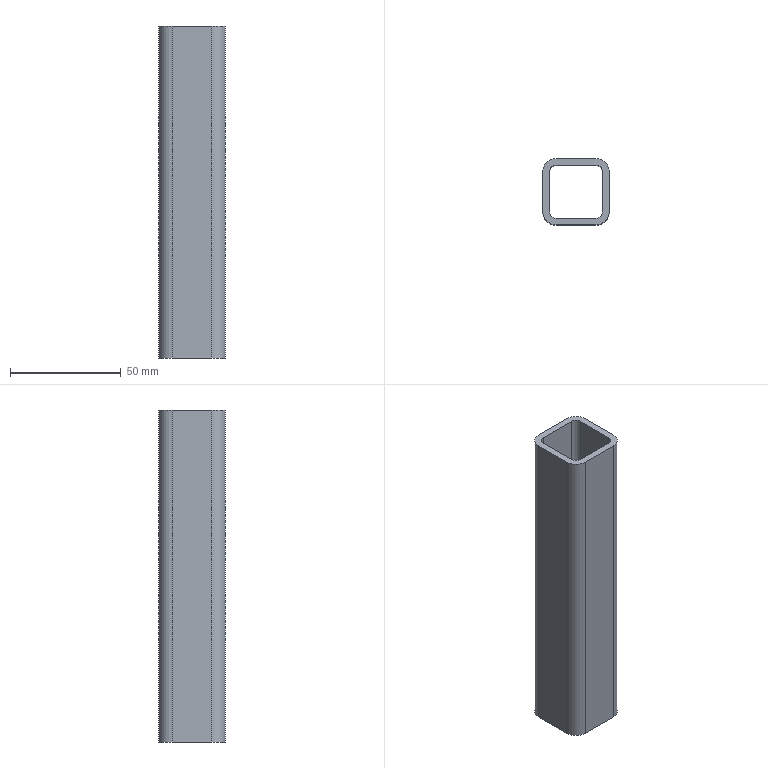Part | NX | features DATUM_CSYS 2, EXTRUDE 1, SKETCH 1 | 1 solid | 18 faces | box 30 x 30 x 150 mm | volume 45123 mm3 | plane 10 | cylinder 8 | commonest cylinder face diameters 6 x4 12 x4
STEP:
#1=CARTESIAN_POINT('',(15.,9.,150.));
#2=VERTEX_POINT('',#1);
#3=CARTESIAN_POINT('',(9.,15.,150.));
#4=VERTEX_POINT('',#3);
#5=CARTESIAN_POINT('',(9.,9.,150.));
#6=DIRECTION('',(0.,0.,1.));
#7=DIRECTION('',(1.,0.,0.));
#8=AXIS2_PLACEMENT_3D('',#5,#6,#7);
#9=CIRCLE('',#8,6.);
#10=EDGE_CURVE('',#2,#4,#9,.T.);
#11=ORIENTED_EDGE('',*,*,#10,.T.);
#12=CARTESIAN_POINT('',(-9.,15.,150.));
#13=VERTEX_POINT('',#12);
#14=CARTESIAN_POINT('',(9.,15.,150.));
#15=DIRECTION('',(-1.,0.,0.));
#16=VECTOR('',#15,1000.);
#17=LINE('',#14,#16);
#18=EDGE_CURVE('',#4,#13,#17,.T.);
#19=ORIENTED_EDGE('',*,*,#18,.T.);
#20=CARTESIAN_POINT('',(-15.,9.,150.));
#21=VERTEX_POINT('',#20);
#22=CARTESIAN_POINT('',(-9.,9.,150.));
#23=DIRECTION('',(0.,0.,1.));
#24=DIRECTION('',(1.,0.,0.));
#25=AXIS2_PLACEMENT_3D('',#22,#23,#24);
#26=CIRCLE('',#25,6.);
#27=EDGE_CURVE('',#13,#21,#26,.T.);
#28=ORIENTED_EDGE('',*,*,#27,.T.);
#29=CARTESIAN_POINT('',(-15.,-9.,150.));
#30=VERTEX_POINT('',#29);
#31=CARTESIAN_POINT('',(-15.,9.,150.));
#32=DIRECTION('',(0.,-1.,0.));
#33=VECTOR('',#32,1000.);
#34=LINE('',#31,#33);
#35=EDGE_CURVE('',#21,#30,#34,.T.);
#36=ORIENTED_EDGE('',*,*,#35,.T.);
#37=CARTESIAN_POINT('',(-9.,-15.,150.));
#38=VERTEX_POINT('',#37);
#39=CARTESIAN_POINT('',(-9.,-9.,150.));
#40=DIRECTION('',(0.,0.,1.));
#41=DIRECTION('',(1.,0.,0.));
#42=AXIS2_PLACEMENT_3D('',#39,#40,#41);
#43=CIRCLE('',#42,6.);
#44=EDGE_CURVE('',#30,#38,#43,.T.);
#45=ORIENTED_EDGE('',*,*,#44,.T.);
#46=CARTESIAN_POINT('',(9.,-15.,150.));
#47=VERTEX_POINT('',#46);
#48=CARTESIAN_POINT('',(-9.,-15.,150.));
#49=DIRECTION('',(1.,0.,0.));
#50=VECTOR('',#49,1000.);
#51=LINE('',#48,#50);
#52=EDGE_CURVE('',#38,#47,#51,.T.);
#53=ORIENTED_EDGE('',*,*,#52,.T.);
#54=CARTESIAN_POINT('',(15.,-9.,150.));
#55=VERTEX_POINT('',#54);
#56=CARTESIAN_POINT('',(9.,-9.,150.));
#57=DIRECTION('',(0.,0.,1.));
#58=DIRECTION('',(1.,0.,0.));
#59=AXIS2_PLACEMENT_3D('',#56,#57,#58);
#60=CIRCLE('',#59,6.);
#61=EDGE_CURVE('',#47,#55,#60,.T.);
#62=ORIENTED_EDGE('',*,*,#61,.T.);
#63=CARTESIAN_POINT('',(15.,-9.,150.));
#64=DIRECTION('',(0.,1.,0.));
#65=VECTOR('',#64,1000.);
#66=LINE('',#63,#65);
#67=EDGE_CURVE('',#55,#2,#66,.T.);
#68=ORIENTED_EDGE('',*,*,#67,.T.);
#69=EDGE_LOOP('',(#11,#19,#28,#36,#45,#53,#62,#68));
#70=FACE_BOUND('',#69,.T.);
#71=CARTESIAN_POINT('',(12.,9.,150.));
#72=VERTEX_POINT('',#71);
#73=CARTESIAN_POINT('',(9.,12.,150.));
#74=VERTEX_POINT('',#73);
#75=CARTESIAN_POINT('',(9.,9.,150.));
#76=DIRECTION('',(0.,0.,1.));
#77=DIRECTION('',(1.,0.,0.));
#78=AXIS2_PLACEMENT_3D('',#75,#76,#77);
#79=CIRCLE('',#78,3.);
#80=EDGE_CURVE('',#72,#74,#79,.T.);
#81=ORIENTED_EDGE('',*,*,#80,.F.);
#82=CARTESIAN_POINT('',(12.,-9.,150.));
#83=VERTEX_POINT('',#82);
#84=CARTESIAN_POINT('',(12.,-9.,150.));
#85=DIRECTION('',(0.,1.,0.));
#86=VECTOR('',#85,1000.);
#87=LINE('',#84,#86);
#88=EDGE_CURVE('',#83,#72,#87,.T.);
#89=ORIENTED_EDGE('',*,*,#88,.F.);
#90=CARTESIAN_POINT('',(9.,-12.,150.));
#91=VERTEX_POINT('',#90);
#92=CARTESIAN_POINT('',(9.,-9.,150.));
#93=DIRECTION('',(0.,0.,1.));
#94=DIRECTION('',(1.,0.,0.));
#95=AXIS2_PLACEMENT_3D('',#92,#93,#94);
#96=CIRCLE('',#95,3.);
#97=EDGE_CURVE('',#91,#83,#96,.T.);
#98=ORIENTED_EDGE('',*,*,#97,.F.);
#99=CARTESIAN_POINT('',(-9.,-12.,150.));
#100=VERTEX_POINT('',#99);
#101=CARTESIAN_POINT('',(-9.,-12.,150.));
#102=DIRECTION('',(1.,0.,0.));
#103=VECTOR('',#102,1000.);
#104=LINE('',#101,#103);
#105=EDGE_CURVE('',#100,#91,#104,.T.);
#106=ORIENTED_EDGE('',*,*,#105,.F.);
#107=CARTESIAN_POINT('',(-12.,-9.,150.));
#108=VERTEX_POINT('',#107);
#109=CARTESIAN_POINT('',(-9.,-9.,150.));
#110=DIRECTION('',(0.,0.,1.));
#111=DIRECTION('',(1.,0.,0.));
#112=AXIS2_PLACEMENT_3D('',#109,#110,#111);
#113=CIRCLE('',#112,3.);
#114=EDGE_CURVE('',#108,#100,#113,.T.);
#115=ORIENTED_EDGE('',*,*,#114,.F.);
#116=CARTESIAN_POINT('',(-12.,9.,150.));
#117=VERTEX_POINT('',#116);
#118=CARTESIAN_POINT('',(-12.,9.,150.));
#119=DIRECTION('',(0.,1.,0.));
#120=VECTOR('',#119,1000.);
#121=LINE('',#118,#120);
#122=EDGE_CURVE('',#117,#108,#121,.F.);
#123=ORIENTED_EDGE('',*,*,#122,.F.);
#124=CARTESIAN_POINT('',(-9.,12.,150.));
#125=VERTEX_POINT('',#124);
#126=CARTESIAN_POINT('',(-9.,9.,150.));
#127=DIRECTION('',(0.,0.,1.));
#128=DIRECTION('',(1.,0.,0.));
#129=AXIS2_PLACEMENT_3D('',#126,#127,#128);
#130=CIRCLE('',#129,3.);
#131=EDGE_CURVE('',#125,#117,#130,.T.);
#132=ORIENTED_EDGE('',*,*,#131,.F.);
#133=CARTESIAN_POINT('',(9.,12.,150.));
#134=DIRECTION('',(-1.,0.,0.));
#135=VECTOR('',#134,1000.);
#136=LINE('',#133,#135);
#137=EDGE_CURVE('',#74,#125,#136,.T.);
#138=ORIENTED_EDGE('',*,*,#137,.F.);
#139=EDGE_LOOP('',(#81,#89,#98,#106,#115,#123,#132,#138));
#140=FACE_BOUND('',#139,.T.);
#141=CARTESIAN_POINT('',(9.,9.,150.));
#142=DIRECTION('',(0.,0.,-1.));
#143=DIRECTION('',(-1.,0.,0.));
#144=AXIS2_PLACEMENT_3D('',#141,#142,#143);
#145=PLANE('',#144);
#146=ADVANCED_FACE('',(#70,#140),#145,.F.);
#147=CARTESIAN_POINT('',(-9.,15.,0.));
#148=VERTEX_POINT('',#147);
#149=CARTESIAN_POINT('',(-15.,9.,0.));
#150=VERTEX_POINT('',#149);
#151=CARTESIAN_POINT('',(-9.,9.,0.));
#152=DIRECTION('',(0.,0.,1.));
#153=DIRECTION('',(1.,0.,0.));
#154=AXIS2_PLACEMENT_3D('',#151,#152,#153);
#155=CIRCLE('',#154,6.);
#156=EDGE_CURVE('',#148,#150,#155,.T.);
#157=ORIENTED_EDGE('',*,*,#156,.F.);
#158=CARTESIAN_POINT('',(9.,15.,0.));
#159=VERTEX_POINT('',#158);
#160=CARTESIAN_POINT('',(9.,15.,0.));
#161=DIRECTION('',(-1.,0.,0.));
#162=VECTOR('',#161,1000.);
#163=LINE('',#160,#162);
#164=EDGE_CURVE('',#159,#148,#163,.T.);
#165=ORIENTED_EDGE('',*,*,#164,.F.);
#166=CARTESIAN_POINT('',(15.,9.,0.));
#167=VERTEX_POINT('',#166);
#168=CARTESIAN_POINT('',(9.,9.,0.));
#169=DIRECTION('',(0.,0.,1.));
#170=DIRECTION('',(1.,0.,0.));
#171=AXIS2_PLACEMENT_3D('',#168,#169,#170);
#172=CIRCLE('',#171,6.);
#173=EDGE_CURVE('',#167,#159,#172,.T.);
#174=ORIENTED_EDGE('',*,*,#173,.F.);
#175=CARTESIAN_POINT('',(15.,-9.,0.));
#176=VERTEX_POINT('',#175);
#177=CARTESIAN_POINT('',(15.,-9.,0.));
#178=DIRECTION('',(0.,1.,0.));
#179=VECTOR('',#178,1000.);
#180=LINE('',#177,#179);
#181=EDGE_CURVE('',#176,#167,#180,.T.);
#182=ORIENTED_EDGE('',*,*,#181,.F.);
#183=CARTESIAN_POINT('',(9.,-15.,0.));
#184=VERTEX_POINT('',#183);
#185=CARTESIAN_POINT('',(9.,-9.,0.));
#186=DIRECTION('',(0.,0.,1.));
#187=DIRECTION('',(1.,0.,0.));
#188=AXIS2_PLACEMENT_3D('',#185,#186,#187);
#189=CIRCLE('',#188,6.);
#190=EDGE_CURVE('',#184,#176,#189,.T.);
#191=ORIENTED_EDGE('',*,*,#190,.F.);
#192=CARTESIAN_POINT('',(-9.,-15.,0.));
#193=VERTEX_POINT('',#192);
#194=CARTESIAN_POINT('',(-9.,-15.,0.));
#195=DIRECTION('',(1.,0.,0.));
#196=VECTOR('',#195,1000.);
#197=LINE('',#194,#196);
#198=EDGE_CURVE('',#193,#184,#197,.T.);
#199=ORIENTED_EDGE('',*,*,#198,.F.);
#200=CARTESIAN_POINT('',(-15.,-9.,0.));
#201=VERTEX_POINT('',#200);
#202=CARTESIAN_POINT('',(-9.,-9.,0.));
#203=DIRECTION('',(0.,0.,1.));
#204=DIRECTION('',(1.,0.,0.));
#205=AXIS2_PLACEMENT_3D('',#202,#203,#204);
#206=CIRCLE('',#205,6.);
#207=EDGE_CURVE('',#201,#193,#206,.T.);
#208=ORIENTED_EDGE('',*,*,#207,.F.);
#209=CARTESIAN_POINT('',(-15.,9.,0.));
#210=DIRECTION('',(0.,-1.,0.));
#211=VECTOR('',#210,1000.);
#212=LINE('',#209,#211);
#213=EDGE_CURVE('',#150,#201,#212,.T.);
#214=ORIENTED_EDGE('',*,*,#213,.F.);
#215=EDGE_LOOP('',(#157,#165,#174,#182,#191,#199,#208,#214));
#216=FACE_BOUND('',#215,.T.);
#217=CARTESIAN_POINT('',(-9.,12.,0.));
#218=VERTEX_POINT('',#217);
#219=CARTESIAN_POINT('',(-12.,9.,0.));
#220=VERTEX_POINT('',#219);
#221=CARTESIAN_POINT('',(-9.,9.,0.));
#222=DIRECTION('',(0.,0.,1.));
#223=DIRECTION('',(1.,0.,0.));
#224=AXIS2_PLACEMENT_3D('',#221,#222,#223);
#225=CIRCLE('',#224,3.);
#226=EDGE_CURVE('',#218,#220,#225,.T.);
#227=ORIENTED_EDGE('',*,*,#226,.T.);
#228=CARTESIAN_POINT('',(-12.,-9.,0.));
#229=VERTEX_POINT('',#228);
#230=CARTESIAN_POINT('',(-12.,9.,0.));
#231=DIRECTION('',(0.,1.,0.));
#232=VECTOR('',#231,1000.);
#233=LINE('',#230,#232);
#234=EDGE_CURVE('',#220,#229,#233,.F.);
#235=ORIENTED_EDGE('',*,*,#234,.T.);
#236=CARTESIAN_POINT('',(-9.,-12.,0.));
#237=VERTEX_POINT('',#236);
#238=CARTESIAN_POINT('',(-9.,-9.,0.));
#239=DIRECTION('',(0.,0.,1.));
#240=DIRECTION('',(1.,0.,0.));
#241=AXIS2_PLACEMENT_3D('',#238,#239,#240);
#242=CIRCLE('',#241,3.);
#243=EDGE_CURVE('',#229,#237,#242,.T.);
#244=ORIENTED_EDGE('',*,*,#243,.T.);
#245=CARTESIAN_POINT('',(9.,-12.,0.));
#246=VERTEX_POINT('',#245);
#247=CARTESIAN_POINT('',(-9.,-12.,0.));
#248=DIRECTION('',(1.,0.,0.));
#249=VECTOR('',#248,1000.);
#250=LINE('',#247,#249);
#251=EDGE_CURVE('',#237,#246,#250,.T.);
#252=ORIENTED_EDGE('',*,*,#251,.T.);
#253=CARTESIAN_POINT('',(12.,-9.,0.));
#254=VERTEX_POINT('',#253);
#255=CARTESIAN_POINT('',(9.,-9.,0.));
#256=DIRECTION('',(0.,0.,1.));
#257=DIRECTION('',(1.,0.,0.));
#258=AXIS2_PLACEMENT_3D('',#255,#256,#257);
#259=CIRCLE('',#258,3.);
#260=EDGE_CURVE('',#246,#254,#259,.T.);
#261=ORIENTED_EDGE('',*,*,#260,.T.);
#262=CARTESIAN_POINT('',(12.,9.,0.));
#263=VERTEX_POINT('',#262);
#264=CARTESIAN_POINT('',(12.,-9.,0.));
#265=DIRECTION('',(0.,1.,0.));
#266=VECTOR('',#265,1000.);
#267=LINE('',#264,#266);
#268=EDGE_CURVE('',#254,#263,#267,.T.);
#269=ORIENTED_EDGE('',*,*,#268,.T.);
#270=CARTESIAN_POINT('',(9.,12.,0.));
#271=VERTEX_POINT('',#270);
#272=CARTESIAN_POINT('',(9.,9.,0.));
#273=DIRECTION('',(0.,0.,1.));
#274=DIRECTION('',(1.,0.,0.));
#275=AXIS2_PLACEMENT_3D('',#272,#273,#274);
#276=CIRCLE('',#275,3.);
#277=EDGE_CURVE('',#263,#271,#276,.T.);
#278=ORIENTED_EDGE('',*,*,#277,.T.);
#279=CARTESIAN_POINT('',(9.,12.,0.));
#280=DIRECTION('',(-1.,0.,0.));
#281=VECTOR('',#280,1000.);
#282=LINE('',#279,#281);
#283=EDGE_CURVE('',#271,#218,#282,.T.);
#284=ORIENTED_EDGE('',*,*,#283,.T.);
#285=EDGE_LOOP('',(#227,#235,#244,#252,#261,#269,#278,#284));
#286=FACE_BOUND('',#285,.T.);
#287=CARTESIAN_POINT('',(-9.,9.,0.));
#288=DIRECTION('',(0.,0.,-1.));
#289=DIRECTION('',(-1.,0.,0.));
#290=AXIS2_PLACEMENT_3D('',#287,#288,#289);
#291=PLANE('',#290);
#292=ADVANCED_FACE('',(#216,#286),#291,.T.);
#293=ORIENTED_EDGE('',*,*,#18,.F.);
#294=CARTESIAN_POINT('',(9.,15.,0.));
#295=DIRECTION('',(0.,0.,1.));
#296=VECTOR('',#295,1000.);
#297=LINE('',#294,#296);
#298=EDGE_CURVE('',#159,#4,#297,.T.);
#299=ORIENTED_EDGE('',*,*,#298,.F.);
#300=ORIENTED_EDGE('',*,*,#164,.T.);
#301=CARTESIAN_POINT('',(-9.,15.,0.));
#302=DIRECTION('',(0.,0.,1.));
#303=VECTOR('',#302,1000.);
#304=LINE('',#301,#303);
#305=EDGE_CURVE('',#148,#13,#304,.T.);
#306=ORIENTED_EDGE('',*,*,#305,.T.);
#307=EDGE_LOOP('',(#293,#299,#300,#306));
#308=FACE_BOUND('',#307,.T.);
#309=CARTESIAN_POINT('',(9.,15.,0.));
#310=DIRECTION('',(0.,1.,0.));
#311=DIRECTION('',(-1.,0.,0.));
#312=AXIS2_PLACEMENT_3D('',#309,#310,#311);
#313=PLANE('',#312);
#314=ADVANCED_FACE('',(#308),#313,.T.);
#315=ORIENTED_EDGE('',*,*,#27,.F.);
#316=ORIENTED_EDGE('',*,*,#305,.F.);
#317=ORIENTED_EDGE('',*,*,#156,.T.);
#318=CARTESIAN_POINT('',(-15.,9.,0.));
#319=DIRECTION('',(0.,0.,1.));
#320=VECTOR('',#319,1000.);
#321=LINE('',#318,#320);
#322=EDGE_CURVE('',#150,#21,#321,.T.);
#323=ORIENTED_EDGE('',*,*,#322,.T.);
#324=EDGE_LOOP('',(#315,#316,#317,#323));
#325=FACE_BOUND('',#324,.T.);
#326=CARTESIAN_POINT('',(-9.,9.,0.));
#327=DIRECTION('',(0.,0.,1.));
#328=DIRECTION('',(1.,0.,0.));
#329=AXIS2_PLACEMENT_3D('',#326,#327,#328);
#330=CYLINDRICAL_SURFACE('',#329,6.);
#331=ADVANCED_FACE('',(#325),#330,.T.);
#332=ORIENTED_EDGE('',*,*,#35,.F.);
#333=ORIENTED_EDGE('',*,*,#322,.F.);
#334=ORIENTED_EDGE('',*,*,#213,.T.);
#335=CARTESIAN_POINT('',(-15.,-9.,0.));
#336=DIRECTION('',(0.,0.,1.));
#337=VECTOR('',#336,1000.);
#338=LINE('',#335,#337);
#339=EDGE_CURVE('',#201,#30,#338,.T.);
#340=ORIENTED_EDGE('',*,*,#339,.T.);
#341=EDGE_LOOP('',(#332,#333,#334,#340));
#342=FACE_BOUND('',#341,.T.);
#343=CARTESIAN_POINT('',(-15.,9.,0.));
#344=DIRECTION('',(-1.,0.,0.));
#345=DIRECTION('',(0.,0.,1.));
#346=AXIS2_PLACEMENT_3D('',#343,#344,#345);
#347=PLANE('',#346);
#348=ADVANCED_FACE('',(#342),#347,.T.);
#349=ORIENTED_EDGE('',*,*,#44,.F.);
#350=ORIENTED_EDGE('',*,*,#339,.F.);
#351=ORIENTED_EDGE('',*,*,#207,.T.);
#352=CARTESIAN_POINT('',(-9.,-15.,0.));
#353=DIRECTION('',(0.,0.,1.));
#354=VECTOR('',#353,1000.);
#355=LINE('',#352,#354);
#356=EDGE_CURVE('',#193,#38,#355,.T.);
#357=ORIENTED_EDGE('',*,*,#356,.T.);
#358=EDGE_LOOP('',(#349,#350,#351,#357));
#359=FACE_BOUND('',#358,.T.);
#360=CARTESIAN_POINT('',(-9.,-9.,0.));
#361=DIRECTION('',(0.,0.,1.));
#362=DIRECTION('',(1.,0.,0.));
#363=AXIS2_PLACEMENT_3D('',#360,#361,#362);
#364=CYLINDRICAL_SURFACE('',#363,6.);
#365=ADVANCED_FACE('',(#359),#364,.T.);
#366=ORIENTED_EDGE('',*,*,#52,.F.);
#367=ORIENTED_EDGE('',*,*,#356,.F.);
#368=ORIENTED_EDGE('',*,*,#198,.T.);
#369=CARTESIAN_POINT('',(9.,-15.,0.));
#370=DIRECTION('',(0.,0.,1.));
#371=VECTOR('',#370,1000.);
#372=LINE('',#369,#371);
#373=EDGE_CURVE('',#184,#47,#372,.T.);
#374=ORIENTED_EDGE('',*,*,#373,.T.);
#375=EDGE_LOOP('',(#366,#367,#368,#374));
#376=FACE_BOUND('',#375,.T.);
#377=CARTESIAN_POINT('',(-9.,-15.,0.));
#378=DIRECTION('',(0.,-1.,0.));
#379=DIRECTION('',(1.,0.,0.));
#380=AXIS2_PLACEMENT_3D('',#377,#378,#379);
#381=PLANE('',#380);
#382=ADVANCED_FACE('',(#376),#381,.T.);
#383=ORIENTED_EDGE('',*,*,#61,.F.);
#384=ORIENTED_EDGE('',*,*,#373,.F.);
#385=ORIENTED_EDGE('',*,*,#190,.T.);
#386=CARTESIAN_POINT('',(15.,-9.,0.));
#387=DIRECTION('',(0.,0.,1.));
#388=VECTOR('',#387,1000.);
#389=LINE('',#386,#388);
#390=EDGE_CURVE('',#176,#55,#389,.T.);
#391=ORIENTED_EDGE('',*,*,#390,.T.);
#392=EDGE_LOOP('',(#383,#384,#385,#391));
#393=FACE_BOUND('',#392,.T.);
#394=CARTESIAN_POINT('',(9.,-9.,0.));
#395=DIRECTION('',(0.,0.,1.));
#396=DIRECTION('',(1.,0.,0.));
#397=AXIS2_PLACEMENT_3D('',#394,#395,#396);
#398=CYLINDRICAL_SURFACE('',#397,6.);
#399=ADVANCED_FACE('',(#393),#398,.T.);
#400=ORIENTED_EDGE('',*,*,#67,.F.);
#401=ORIENTED_EDGE('',*,*,#390,.F.);
#402=ORIENTED_EDGE('',*,*,#181,.T.);
#403=CARTESIAN_POINT('',(15.,9.,0.));
#404=DIRECTION('',(0.,0.,1.));
#405=VECTOR('',#404,1000.);
#406=LINE('',#403,#405);
#407=EDGE_CURVE('',#167,#2,#406,.T.);
#408=ORIENTED_EDGE('',*,*,#407,.T.);
#409=EDGE_LOOP('',(#400,#401,#402,#408));
#410=FACE_BOUND('',#409,.T.);
#411=CARTESIAN_POINT('',(15.,-9.,0.));
#412=DIRECTION('',(1.,0.,0.));
#413=DIRECTION('',(0.,0.,-1.));
#414=AXIS2_PLACEMENT_3D('',#411,#412,#413);
#415=PLANE('',#414);
#416=ADVANCED_FACE('',(#410),#415,.T.);
#417=ORIENTED_EDGE('',*,*,#10,.F.);
#418=ORIENTED_EDGE('',*,*,#407,.F.);
#419=ORIENTED_EDGE('',*,*,#173,.T.);
#420=ORIENTED_EDGE('',*,*,#298,.T.);
#421=EDGE_LOOP('',(#417,#418,#419,#420));
#422=FACE_BOUND('',#421,.T.);
#423=CARTESIAN_POINT('',(9.,9.,0.));
#424=DIRECTION('',(0.,0.,1.));
#425=DIRECTION('',(1.,0.,0.));
#426=AXIS2_PLACEMENT_3D('',#423,#424,#425);
#427=CYLINDRICAL_SURFACE('',#426,6.);
#428=ADVANCED_FACE('',(#422),#427,.T.);
#429=ORIENTED_EDGE('',*,*,#137,.T.);
#430=CARTESIAN_POINT('',(-9.,12.,0.));
#431=DIRECTION('',(0.,0.,1.));
#432=VECTOR('',#431,1000.);
#433=LINE('',#430,#432);
#434=EDGE_CURVE('',#218,#125,#433,.T.);
#435=ORIENTED_EDGE('',*,*,#434,.F.);
#436=ORIENTED_EDGE('',*,*,#283,.F.);
#437=CARTESIAN_POINT('',(9.,12.,0.));
#438=DIRECTION('',(0.,0.,1.));
#439=VECTOR('',#438,1000.);
#440=LINE('',#437,#439);
#441=EDGE_CURVE('',#271,#74,#440,.T.);
#442=ORIENTED_EDGE('',*,*,#441,.T.);
#443=EDGE_LOOP('',(#429,#435,#436,#442));
#444=FACE_BOUND('',#443,.T.);
#445=CARTESIAN_POINT('',(9.,12.,0.));
#446=DIRECTION('',(0.,1.,0.));
#447=DIRECTION('',(-1.,0.,0.));
#448=AXIS2_PLACEMENT_3D('',#445,#446,#447);
#449=PLANE('',#448);
#450=ADVANCED_FACE('',(#444),#449,.F.);
#451=ORIENTED_EDGE('',*,*,#131,.T.);
#452=CARTESIAN_POINT('',(-12.,9.,0.));
#453=DIRECTION('',(0.,0.,1.));
#454=VECTOR('',#453,1000.);
#455=LINE('',#452,#454);
#456=EDGE_CURVE('',#220,#117,#455,.T.);
#457=ORIENTED_EDGE('',*,*,#456,.F.);
#458=ORIENTED_EDGE('',*,*,#226,.F.);
#459=ORIENTED_EDGE('',*,*,#434,.T.);
#460=EDGE_LOOP('',(#451,#457,#458,#459));
#461=FACE_BOUND('',#460,.T.);
#462=CARTESIAN_POINT('',(-9.,9.,0.));
#463=DIRECTION('',(0.,0.,1.));
#464=DIRECTION('',(1.,0.,0.));
#465=AXIS2_PLACEMENT_3D('',#462,#463,#464);
#466=CYLINDRICAL_SURFACE('',#465,3.);
#467=ADVANCED_FACE('',(#461),#466,.F.);
#468=ORIENTED_EDGE('',*,*,#122,.T.);
#469=CARTESIAN_POINT('',(-12.,-9.,0.));
#470=DIRECTION('',(0.,0.,1.));
#471=VECTOR('',#470,1000.);
#472=LINE('',#469,#471);
#473=EDGE_CURVE('',#229,#108,#472,.T.);
#474=ORIENTED_EDGE('',*,*,#473,.F.);
#475=ORIENTED_EDGE('',*,*,#234,.F.);
#476=ORIENTED_EDGE('',*,*,#456,.T.);
#477=EDGE_LOOP('',(#468,#474,#475,#476));
#478=FACE_BOUND('',#477,.T.);
#479=CARTESIAN_POINT('',(-12.,9.,0.));
#480=DIRECTION('',(-1.,0.,0.));
#481=DIRECTION('',(0.,0.,1.));
#482=AXIS2_PLACEMENT_3D('',#479,#480,#481);
#483=PLANE('',#482);
#484=ADVANCED_FACE('',(#478),#483,.F.);
#485=ORIENTED_EDGE('',*,*,#114,.T.);
#486=CARTESIAN_POINT('',(-9.,-12.,0.));
#487=DIRECTION('',(0.,0.,1.));
#488=VECTOR('',#487,1000.);
#489=LINE('',#486,#488);
#490=EDGE_CURVE('',#237,#100,#489,.T.);
#491=ORIENTED_EDGE('',*,*,#490,.F.);
#492=ORIENTED_EDGE('',*,*,#243,.F.);
#493=ORIENTED_EDGE('',*,*,#473,.T.);
#494=EDGE_LOOP('',(#485,#491,#492,#493));
#495=FACE_BOUND('',#494,.T.);
#496=CARTESIAN_POINT('',(-9.,-9.,0.));
#497=DIRECTION('',(0.,0.,1.));
#498=DIRECTION('',(1.,0.,0.));
#499=AXIS2_PLACEMENT_3D('',#496,#497,#498);
#500=CYLINDRICAL_SURFACE('',#499,3.);
#501=ADVANCED_FACE('',(#495),#500,.F.);
#502=ORIENTED_EDGE('',*,*,#105,.T.);
#503=CARTESIAN_POINT('',(9.,-12.,0.));
#504=DIRECTION('',(0.,0.,1.));
#505=VECTOR('',#504,1000.);
#506=LINE('',#503,#505);
#507=EDGE_CURVE('',#246,#91,#506,.T.);
#508=ORIENTED_EDGE('',*,*,#507,.F.);
#509=ORIENTED_EDGE('',*,*,#251,.F.);
#510=ORIENTED_EDGE('',*,*,#490,.T.);
#511=EDGE_LOOP('',(#502,#508,#509,#510));
#512=FACE_BOUND('',#511,.T.);
#513=CARTESIAN_POINT('',(-9.,-12.,0.));
#514=DIRECTION('',(0.,-1.,0.));
#515=DIRECTION('',(1.,0.,0.));
#516=AXIS2_PLACEMENT_3D('',#513,#514,#515);
#517=PLANE('',#516);
#518=ADVANCED_FACE('',(#512),#517,.F.);
#519=ORIENTED_EDGE('',*,*,#97,.T.);
#520=CARTESIAN_POINT('',(12.,-9.,0.));
#521=DIRECTION('',(0.,0.,1.));
#522=VECTOR('',#521,1000.);
#523=LINE('',#520,#522);
#524=EDGE_CURVE('',#254,#83,#523,.T.);
#525=ORIENTED_EDGE('',*,*,#524,.F.);
#526=ORIENTED_EDGE('',*,*,#260,.F.);
#527=ORIENTED_EDGE('',*,*,#507,.T.);
#528=EDGE_LOOP('',(#519,#525,#526,#527));
#529=FACE_BOUND('',#528,.T.);
#530=CARTESIAN_POINT('',(9.,-9.,0.));
#531=DIRECTION('',(0.,0.,1.));
#532=DIRECTION('',(1.,0.,0.));
#533=AXIS2_PLACEMENT_3D('',#530,#531,#532);
#534=CYLINDRICAL_SURFACE('',#533,3.);
#535=ADVANCED_FACE('',(#529),#534,.F.);
#536=ORIENTED_EDGE('',*,*,#88,.T.);
#537=CARTESIAN_POINT('',(12.,9.,0.));
#538=DIRECTION('',(0.,0.,-1.));
#539=VECTOR('',#538,1000.);
#540=LINE('',#537,#539);
#541=EDGE_CURVE('',#263,#72,#540,.F.);
#542=ORIENTED_EDGE('',*,*,#541,.F.);
#543=ORIENTED_EDGE('',*,*,#268,.F.);
#544=ORIENTED_EDGE('',*,*,#524,.T.);
#545=EDGE_LOOP('',(#536,#542,#543,#544));
#546=FACE_BOUND('',#545,.T.);
#547=CARTESIAN_POINT('',(12.,-9.,0.));
#548=DIRECTION('',(1.,0.,0.));
#549=DIRECTION('',(0.,0.,-1.));
#550=AXIS2_PLACEMENT_3D('',#547,#548,#549);
#551=PLANE('',#550);
#552=ADVANCED_FACE('',(#546),#551,.F.);
#553=ORIENTED_EDGE('',*,*,#80,.T.);
#554=ORIENTED_EDGE('',*,*,#441,.F.);
#555=ORIENTED_EDGE('',*,*,#277,.F.);
#556=ORIENTED_EDGE('',*,*,#541,.T.);
#557=EDGE_LOOP('',(#553,#554,#555,#556));
#558=FACE_BOUND('',#557,.T.);
#559=CARTESIAN_POINT('',(9.,9.,0.));
#560=DIRECTION('',(0.,0.,1.));
#561=DIRECTION('',(1.,0.,0.));
#562=AXIS2_PLACEMENT_3D('',#559,#560,#561);
#563=CYLINDRICAL_SURFACE('',#562,3.);
#564=ADVANCED_FACE('',(#558),#563,.F.);
#565=CLOSED_SHELL('',(#146,#292,#314,#331,#348,#365,#382,#399,#416,#428,#450,#467,#484,#501,#518,#535,#552,#564));
#566=MANIFOLD_SOLID_BREP('',#565);
#567=(LENGTH_UNIT()NAMED_UNIT(*)SI_UNIT(.MILLI.,.METRE.));
#568=UNCERTAINTY_MEASURE_WITH_UNIT(LENGTH_MEASURE(0.00001),#567,'','');
#569=(NAMED_UNIT(*)PLANE_ANGLE_UNIT()SI_UNIT($,.RADIAN.));
#570=(NAMED_UNIT(*)SI_UNIT($,.STERADIAN.)SOLID_ANGLE_UNIT());
#571=(GEOMETRIC_REPRESENTATION_CONTEXT(3)GLOBAL_UNCERTAINTY_ASSIGNED_CONTEXT((#568))GLOBAL_UNIT_ASSIGNED_CONTEXT((#567,#569,#570))REPRESENTATION_CONTEXT('',''));
#572=ADVANCED_BREP_SHAPE_REPRESENTATION('',(#566),#571);